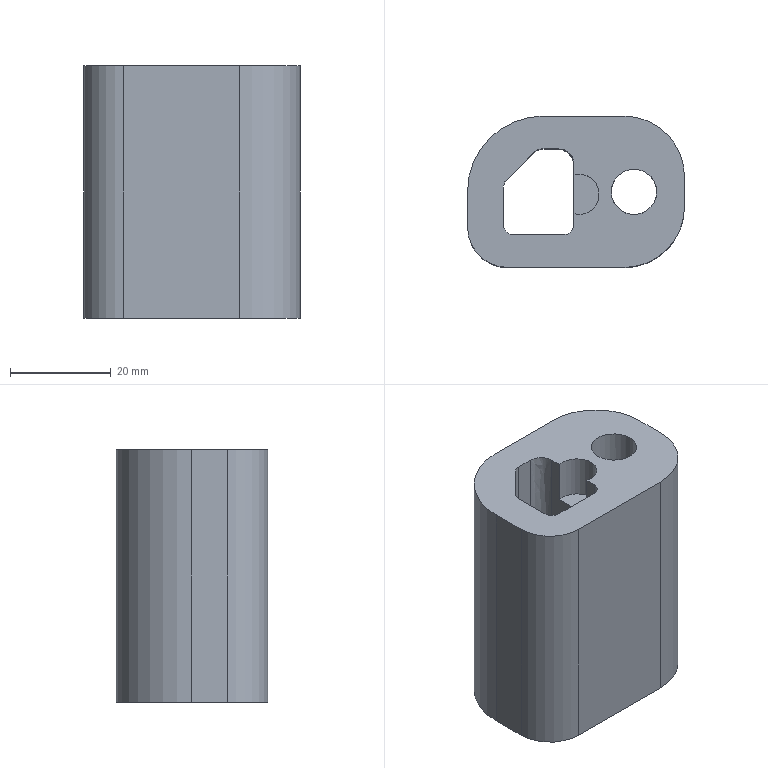Part | STEP file | PN_0018_id894_x_t | 1 solid | 25 faces | box 43 x 30 x 50 mm | volume 41594 mm3 | plane 13 | cylinder 10 | other 2 | commonest cylinder face diameters 4 x3 24 x2 8 x1 9 x1 14 x1 16 x1
STEP:
#1=CARTESIAN_POINT('',(-194.5,-101.127,86.5));
#2=VERTEX_POINT('',#1);
#3=CARTESIAN_POINT('',(-194.5,-108.873,86.5));
#4=VERTEX_POINT('',#3);
#5=CARTESIAN_POINT('',(-194.5,-99.,86.5));
#6=DIRECTION('',(0.,-1.,0.));
#7=VECTOR('',#6,1.);
#8=LINE('',#5,#7);
#9=EDGE_CURVE('',#2,#4,#8,.T.);
#10=ORIENTED_EDGE('',*,*,#9,.F.);
#11=CARTESIAN_POINT('',(-194.5,-101.127,95.));
#12=VERTEX_POINT('',#11);
#13=CARTESIAN_POINT('',(-194.5,-101.127,86.5));
#14=DIRECTION('',(0.,0.,1.));
#15=VECTOR('',#14,1.);
#16=LINE('',#13,#15);
#17=EDGE_CURVE('',#2,#12,#16,.T.);
#18=ORIENTED_EDGE('',*,*,#17,.T.);
#19=CARTESIAN_POINT('',(-194.5,-99.,95.));
#20=VERTEX_POINT('',#19);
#21=CARTESIAN_POINT('',(-194.5,-99.,95.));
#22=DIRECTION('',(0.,-1.,0.));
#23=VECTOR('',#22,1.);
#24=LINE('',#21,#23);
#25=EDGE_CURVE('',#20,#12,#24,.T.);
#26=ORIENTED_EDGE('',*,*,#25,.F.);
#27=CARTESIAN_POINT('',(-194.5,-99.,45.));
#28=VERTEX_POINT('',#27);
#29=CARTESIAN_POINT('',(-194.5,-99.,78.6));
#30=DIRECTION('',(0.,0.,-1.));
#31=VECTOR('',#30,1.);
#32=LINE('',#29,#31);
#33=EDGE_CURVE('',#20,#28,#32,.T.);
#34=ORIENTED_EDGE('',*,*,#33,.T.);
#35=CARTESIAN_POINT('',(-194.5,-111.,45.));
#36=VERTEX_POINT('',#35);
#37=CARTESIAN_POINT('',(-194.5,-99.,45.));
#38=DIRECTION('',(0.,-1.,0.));
#39=VECTOR('',#38,1.);
#40=LINE('',#37,#39);
#41=EDGE_CURVE('',#28,#36,#40,.T.);
#42=ORIENTED_EDGE('',*,*,#41,.T.);
#43=CARTESIAN_POINT('',(-194.5,-111.,95.));
#44=VERTEX_POINT('',#43);
#45=CARTESIAN_POINT('',(-194.5,-111.,78.6));
#46=DIRECTION('',(0.,0.,-1.));
#47=VECTOR('',#46,1.);
#48=LINE('',#45,#47);
#49=EDGE_CURVE('',#44,#36,#48,.T.);
#50=ORIENTED_EDGE('',*,*,#49,.F.);
#51=CARTESIAN_POINT('',(-194.5,-108.873,95.));
#52=VERTEX_POINT('',#51);
#53=CARTESIAN_POINT('',(-194.5,-99.,95.));
#54=DIRECTION('',(0.,-1.,0.));
#55=VECTOR('',#54,1.);
#56=LINE('',#53,#55);
#57=EDGE_CURVE('',#52,#44,#56,.T.);
#58=ORIENTED_EDGE('',*,*,#57,.F.);
#59=CARTESIAN_POINT('',(-194.5,-108.873,86.5));
#60=DIRECTION('',(0.,0.,-1.));
#61=VECTOR('',#60,1.);
#62=LINE('',#59,#61);
#63=EDGE_CURVE('',#52,#4,#62,.T.);
#64=ORIENTED_EDGE('',*,*,#63,.T.);
#65=EDGE_LOOP('',(#10,#18,#26,#34,#42,#50,#58,#64));
#66=FACE_OUTER_BOUND('',#65,.T.);
#67=CARTESIAN_POINT('',(-194.5,-99.,78.6));
#68=DIRECTION('',(1.,0.,0.));
#69=DIRECTION('',(0.,0.,-1.));
#70=AXIS2_PLACEMENT_3D('',#67,#68,#69);
#71=PLANE('',#70);
#72=ADVANCED_FACE('',(#66),#71,.F.);
#73=CARTESIAN_POINT('',(-187.086,-104.5,95.));
#74=VERTEX_POINT('',#73);
#75=CARTESIAN_POINT('',(-182.586,-104.5,95.));
#76=DIRECTION('',(0.,0.,1.));
#77=DIRECTION('',(-1.,0.,0.));
#78=AXIS2_PLACEMENT_3D('',#75,#76,#77);
#79=CIRCLE('',#78,4.5);
#80=EDGE_CURVE('',#74,#74,#79,.T.);
#81=ORIENTED_EDGE('',*,*,#80,.F.);
#82=EDGE_LOOP('',(#81));
#83=FACE_BOUND('',#82,.T.);
#84=CARTESIAN_POINT('',(-193.5,-105.,95.));
#85=DIRECTION('',(0.,0.,1.));
#86=DIRECTION('',(1.,0.,0.));
#87=AXIS2_PLACEMENT_3D('',#84,#85,#86);
#88=CIRCLE('',#87,4.);
#89=EDGE_CURVE('',#52,#12,#88,.T.);
#90=ORIENTED_EDGE('',*,*,#89,.F.);
#91=ORIENTED_EDGE('',*,*,#57,.T.);
#92=CARTESIAN_POINT('',(-196.5,-113.,95.));
#93=VERTEX_POINT('',#92);
#94=CARTESIAN_POINT('',(-196.5,-111.,95.));
#95=DIRECTION('',(0.,0.,-1.));
#96=DIRECTION('',(-1.,0.,0.));
#97=AXIS2_PLACEMENT_3D('',#94,#95,#96);
#98=CIRCLE('',#97,2.);
#99=EDGE_CURVE('',#44,#93,#98,.T.);
#100=ORIENTED_EDGE('',*,*,#99,.T.);
#101=CARTESIAN_POINT('',(-206.5,-113.,95.));
#102=VERTEX_POINT('',#101);
#103=CARTESIAN_POINT('',(-196.5,-113.,95.));
#104=DIRECTION('',(-1.,0.,0.));
#105=VECTOR('',#104,1.);
#106=LINE('',#103,#105);
#107=EDGE_CURVE('',#93,#102,#106,.T.);
#108=ORIENTED_EDGE('',*,*,#107,.T.);
#109=CARTESIAN_POINT('',(-208.5,-111.,95.));
#110=VERTEX_POINT('',#109);
#111=CARTESIAN_POINT('',(-206.5,-111.,95.));
#112=DIRECTION('',(0.,0.,-1.));
#113=DIRECTION('',(-1.,0.,0.));
#114=AXIS2_PLACEMENT_3D('',#111,#112,#113);
#115=CIRCLE('',#114,2.);
#116=EDGE_CURVE('',#102,#110,#115,.T.);
#117=ORIENTED_EDGE('',*,*,#116,.T.);
#118=CARTESIAN_POINT('',(-208.5,-103.657,95.));
#119=VERTEX_POINT('',#118);
#120=CARTESIAN_POINT('',(-208.5,-111.,95.));
#121=DIRECTION('',(0.,1.,0.));
#122=VECTOR('',#121,1.);
#123=LINE('',#120,#122);
#124=EDGE_CURVE('',#110,#119,#123,.T.);
#125=ORIENTED_EDGE('',*,*,#124,.T.);
#126=CARTESIAN_POINT('',(-207.914,-102.243,95.));
#127=VERTEX_POINT('',#126);
#128=CARTESIAN_POINT('',(-206.5,-103.657,95.));
#129=DIRECTION('',(0.,0.,-1.));
#130=DIRECTION('',(-1.,0.,0.));
#131=AXIS2_PLACEMENT_3D('',#128,#129,#130);
#132=CIRCLE('',#131,2.);
#133=EDGE_CURVE('',#119,#127,#132,.T.);
#134=ORIENTED_EDGE('',*,*,#133,.T.);
#135=CARTESIAN_POINT('',(-202.257,-96.586,95.));
#136=VERTEX_POINT('',#135);
#137=CARTESIAN_POINT('',(-207.914,-102.243,95.));
#138=DIRECTION('',(0.7071,0.7071,0.));
#139=VECTOR('',#138,1.);
#140=LINE('',#137,#139);
#141=EDGE_CURVE('',#127,#136,#140,.T.);
#142=ORIENTED_EDGE('',*,*,#141,.T.);
#143=CARTESIAN_POINT('',(-200.843,-96.,95.));
#144=VERTEX_POINT('',#143);
#145=CARTESIAN_POINT('',(-202.257,-96.586,95.));
#146=CARTESIAN_POINT('',(-201.885,-96.213,95.));
#147=CARTESIAN_POINT('',(-201.37,-96.,95.));
#148=CARTESIAN_POINT('',(-200.843,-96.,95.));
#149=B_SPLINE_CURVE_WITH_KNOTS('',3,(#145,#146,#147,#148),.UNSPECIFIED.,.F.,.F.,(4,4),(0.,1.),.UNSPECIFIED.);
#150=EDGE_CURVE('',#136,#144,#149,.T.);
#151=ORIENTED_EDGE('',*,*,#150,.T.);
#152=CARTESIAN_POINT('',(-197.5,-96.,95.));
#153=VERTEX_POINT('',#152);
#154=CARTESIAN_POINT('',(-200.843,-96.,95.));
#155=DIRECTION('',(1.,0.,0.));
#156=VECTOR('',#155,1.);
#157=LINE('',#154,#156);
#158=EDGE_CURVE('',#144,#153,#157,.T.);
#159=ORIENTED_EDGE('',*,*,#158,.T.);
#160=CARTESIAN_POINT('',(-197.5,-96.,95.));
#161=CARTESIAN_POINT('',(-196.717,-96.,95.));
#162=CARTESIAN_POINT('',(-195.94,-96.317,95.));
#163=CARTESIAN_POINT('',(-194.817,-97.441,95.));
#164=CARTESIAN_POINT('',(-194.5,-98.203,95.));
#165=CARTESIAN_POINT('',(-194.5,-99.,95.));
#166=B_SPLINE_CURVE_WITH_KNOTS('',3,(#160,#161,#162,#163,#164,#165),.UNSPECIFIED.,.F.,.F.,(4,2,4),(0.,0.5,1.),.UNSPECIFIED.);
#167=EDGE_CURVE('',#153,#20,#166,.T.);
#168=ORIENTED_EDGE('',*,*,#167,.T.);
#169=ORIENTED_EDGE('',*,*,#25,.T.);
#170=EDGE_LOOP('',(#90,#91,#100,#108,#117,#125,#134,#142,#151,#159,#168,#169));
#171=FACE_BOUND('',#170,.T.);
#172=CARTESIAN_POINT('',(-215.586,-104.5,95.));
#173=VERTEX_POINT('',#172);
#174=CARTESIAN_POINT('',(-215.586,-111.5,95.));
#175=VERTEX_POINT('',#174);
#176=CARTESIAN_POINT('',(-215.586,-80.,95.));
#177=DIRECTION('',(0.,-1.,0.));
#178=VECTOR('',#177,1.);
#179=LINE('',#176,#178);
#180=EDGE_CURVE('',#173,#175,#179,.T.);
#181=ORIENTED_EDGE('',*,*,#180,.T.);
#182=CARTESIAN_POINT('',(-207.586,-119.5,95.));
#183=VERTEX_POINT('',#182);
#184=CARTESIAN_POINT('',(-207.586,-111.5,95.));
#185=DIRECTION('',(0.,0.,1.));
#186=DIRECTION('',(-1.,0.,0.));
#187=AXIS2_PLACEMENT_3D('',#184,#185,#186);
#188=CIRCLE('',#187,8.);
#189=EDGE_CURVE('',#175,#183,#188,.T.);
#190=ORIENTED_EDGE('',*,*,#189,.T.);
#191=CARTESIAN_POINT('',(-184.586,-119.5,95.));
#192=VERTEX_POINT('',#191);
#193=CARTESIAN_POINT('',(-211.586,-119.5,95.));
#194=DIRECTION('',(1.,0.,0.));
#195=VECTOR('',#194,1.);
#196=LINE('',#193,#195);
#197=EDGE_CURVE('',#183,#192,#196,.T.);
#198=ORIENTED_EDGE('',*,*,#197,.T.);
#199=CARTESIAN_POINT('',(-172.586,-107.5,95.));
#200=VERTEX_POINT('',#199);
#201=CARTESIAN_POINT('',(-184.586,-107.5,95.));
#202=DIRECTION('',(0.,0.,1.));
#203=DIRECTION('',(-1.,0.,0.));
#204=AXIS2_PLACEMENT_3D('',#201,#202,#203);
#205=CIRCLE('',#204,12.);
#206=EDGE_CURVE('',#192,#200,#205,.T.);
#207=ORIENTED_EDGE('',*,*,#206,.T.);
#208=CARTESIAN_POINT('',(-172.586,-101.5,95.));
#209=VERTEX_POINT('',#208);
#210=CARTESIAN_POINT('',(-172.586,-115.,95.));
#211=DIRECTION('',(0.,1.,0.));
#212=VECTOR('',#211,1.);
#213=LINE('',#210,#212);
#214=EDGE_CURVE('',#200,#209,#213,.T.);
#215=ORIENTED_EDGE('',*,*,#214,.T.);
#216=CARTESIAN_POINT('',(-184.586,-89.5,95.));
#217=VERTEX_POINT('',#216);
#218=CARTESIAN_POINT('',(-184.586,-101.5,95.));
#219=DIRECTION('',(0.,0.,1.));
#220=DIRECTION('',(-1.,0.,0.));
#221=AXIS2_PLACEMENT_3D('',#218,#219,#220);
#222=CIRCLE('',#221,12.);
#223=EDGE_CURVE('',#209,#217,#222,.T.);
#224=ORIENTED_EDGE('',*,*,#223,.T.);
#225=CARTESIAN_POINT('',(-200.586,-89.5,95.));
#226=VERTEX_POINT('',#225);
#227=CARTESIAN_POINT('',(-189.586,-89.5,95.));
#228=DIRECTION('',(-1.,0.,0.));
#229=VECTOR('',#228,1.);
#230=LINE('',#227,#229);
#231=EDGE_CURVE('',#217,#226,#230,.T.);
#232=ORIENTED_EDGE('',*,*,#231,.T.);
#233=CARTESIAN_POINT('',(-200.586,-104.5,95.));
#234=DIRECTION('',(0.,0.,1.));
#235=DIRECTION('',(-1.,0.,0.));
#236=AXIS2_PLACEMENT_3D('',#233,#234,#235);
#237=CIRCLE('',#236,15.);
#238=EDGE_CURVE('',#226,#173,#237,.T.);
#239=ORIENTED_EDGE('',*,*,#238,.T.);
#240=EDGE_LOOP('',(#181,#190,#198,#207,#215,#224,#232,#239));
#241=FACE_BOUND('',#240,.T.);
#242=CARTESIAN_POINT('',(-114.973,24.687,95.));
#243=DIRECTION('',(0.,0.,-1.));
#244=DIRECTION('',(-1.,0.,0.));
#245=AXIS2_PLACEMENT_3D('',#242,#243,#244);
#246=PLANE('',#245);
#247=ADVANCED_FACE('',(#83,#171,#241),#246,.F.);
#248=CARTESIAN_POINT('',(-215.586,-111.5,45.));
#249=VERTEX_POINT('',#248);
#250=CARTESIAN_POINT('',(-215.586,-104.5,45.));
#251=VERTEX_POINT('',#250);
#252=CARTESIAN_POINT('',(-215.586,-64.,45.));
#253=DIRECTION('',(0.,1.,0.));
#254=VECTOR('',#253,1.);
#255=LINE('',#252,#254);
#256=EDGE_CURVE('',#249,#251,#255,.T.);
#257=ORIENTED_EDGE('',*,*,#256,.F.);
#258=CARTESIAN_POINT('',(-215.586,-111.5,78.6));
#259=DIRECTION('',(0.,0.,1.));
#260=VECTOR('',#259,1.);
#261=LINE('',#258,#260);
#262=EDGE_CURVE('',#249,#175,#261,.T.);
#263=ORIENTED_EDGE('',*,*,#262,.T.);
#264=ORIENTED_EDGE('',*,*,#180,.F.);
#265=CARTESIAN_POINT('',(-215.586,-104.5,78.6));
#266=DIRECTION('',(0.,0.,-1.));
#267=VECTOR('',#266,1.);
#268=LINE('',#265,#267);
#269=EDGE_CURVE('',#173,#251,#268,.T.);
#270=ORIENTED_EDGE('',*,*,#269,.T.);
#271=EDGE_LOOP('',(#257,#263,#264,#270));
#272=FACE_OUTER_BOUND('',#271,.T.);
#273=CARTESIAN_POINT('',(-215.586,-80.,78.6));
#274=DIRECTION('',(1.,0.,0.));
#275=DIRECTION('',(0.,0.,-1.));
#276=AXIS2_PLACEMENT_3D('',#273,#274,#275);
#277=PLANE('',#276);
#278=ADVANCED_FACE('',(#272),#277,.F.);
#279=ORIENTED_EDGE('',*,*,#197,.F.);
#280=CARTESIAN_POINT('',(-207.586,-119.5,45.));
#281=VERTEX_POINT('',#280);
#282=CARTESIAN_POINT('',(-207.586,-119.5,78.6));
#283=DIRECTION('',(0.,0.,-1.));
#284=VECTOR('',#283,1.);
#285=LINE('',#282,#284);
#286=EDGE_CURVE('',#183,#281,#285,.T.);
#287=ORIENTED_EDGE('',*,*,#286,.T.);
#288=CARTESIAN_POINT('',(-184.586,-119.5,45.));
#289=VERTEX_POINT('',#288);
#290=CARTESIAN_POINT('',(-211.586,-119.5,45.));
#291=DIRECTION('',(1.,0.,0.));
#292=VECTOR('',#291,1.);
#293=LINE('',#290,#292);
#294=EDGE_CURVE('',#281,#289,#293,.T.);
#295=ORIENTED_EDGE('',*,*,#294,.T.);
#296=CARTESIAN_POINT('',(-184.586,-119.5,78.6));
#297=DIRECTION('',(0.,0.,1.));
#298=VECTOR('',#297,1.);
#299=LINE('',#296,#298);
#300=EDGE_CURVE('',#289,#192,#299,.T.);
#301=ORIENTED_EDGE('',*,*,#300,.T.);
#302=EDGE_LOOP('',(#279,#287,#295,#301));
#303=FACE_OUTER_BOUND('',#302,.T.);
#304=CARTESIAN_POINT('',(-211.586,-119.5,78.6));
#305=DIRECTION('',(0.,1.,0.));
#306=DIRECTION('',(0.,0.,1.));
#307=AXIS2_PLACEMENT_3D('',#304,#305,#306);
#308=PLANE('',#307);
#309=ADVANCED_FACE('',(#303),#308,.F.);
#310=ORIENTED_EDGE('',*,*,#214,.F.);
#311=CARTESIAN_POINT('',(-172.586,-107.5,45.));
#312=VERTEX_POINT('',#311);
#313=CARTESIAN_POINT('',(-172.586,-107.5,78.6));
#314=DIRECTION('',(0.,0.,-1.));
#315=VECTOR('',#314,1.);
#316=LINE('',#313,#315);
#317=EDGE_CURVE('',#200,#312,#316,.T.);
#318=ORIENTED_EDGE('',*,*,#317,.T.);
#319=CARTESIAN_POINT('',(-172.586,-101.5,45.));
#320=VERTEX_POINT('',#319);
#321=CARTESIAN_POINT('',(-172.586,-115.,45.));
#322=DIRECTION('',(0.,1.,0.));
#323=VECTOR('',#322,1.);
#324=LINE('',#321,#323);
#325=EDGE_CURVE('',#312,#320,#324,.T.);
#326=ORIENTED_EDGE('',*,*,#325,.T.);
#327=CARTESIAN_POINT('',(-172.586,-101.5,78.6));
#328=DIRECTION('',(0.,0.,1.));
#329=VECTOR('',#328,1.);
#330=LINE('',#327,#329);
#331=EDGE_CURVE('',#320,#209,#330,.T.);
#332=ORIENTED_EDGE('',*,*,#331,.T.);
#333=EDGE_LOOP('',(#310,#318,#326,#332));
#334=FACE_OUTER_BOUND('',#333,.T.);
#335=CARTESIAN_POINT('',(-172.586,-115.,78.6));
#336=DIRECTION('',(-1.,0.,0.));
#337=DIRECTION('',(0.,0.,1.));
#338=AXIS2_PLACEMENT_3D('',#335,#336,#337);
#339=PLANE('',#338);
#340=ADVANCED_FACE('',(#334),#339,.F.);
#341=CARTESIAN_POINT('',(-200.586,-89.5,45.));
#342=VERTEX_POINT('',#341);
#343=CARTESIAN_POINT('',(-184.586,-89.5,45.));
#344=VERTEX_POINT('',#343);
#345=CARTESIAN_POINT('',(-119.811,-89.5,45.));
#346=DIRECTION('',(1.,0.,0.));
#347=VECTOR('',#346,1.);
#348=LINE('',#345,#347);
#349=EDGE_CURVE('',#342,#344,#348,.T.);
#350=ORIENTED_EDGE('',*,*,#349,.F.);
#351=CARTESIAN_POINT('',(-200.586,-89.5,78.6));
#352=DIRECTION('',(0.,0.,1.));
#353=VECTOR('',#352,1.);
#354=LINE('',#351,#353);
#355=EDGE_CURVE('',#342,#226,#354,.T.);
#356=ORIENTED_EDGE('',*,*,#355,.T.);
#357=ORIENTED_EDGE('',*,*,#231,.F.);
#358=CARTESIAN_POINT('',(-184.586,-89.5,78.6));
#359=DIRECTION('',(0.,0.,-1.));
#360=VECTOR('',#359,1.);
#361=LINE('',#358,#360);
#362=EDGE_CURVE('',#217,#344,#361,.T.);
#363=ORIENTED_EDGE('',*,*,#362,.T.);
#364=EDGE_LOOP('',(#350,#356,#357,#363));
#365=FACE_OUTER_BOUND('',#364,.T.);
#366=CARTESIAN_POINT('',(-189.586,-89.5,78.6));
#367=DIRECTION('',(0.,-1.,0.));
#368=DIRECTION('',(0.,0.,-1.));
#369=AXIS2_PLACEMENT_3D('',#366,#367,#368);
#370=PLANE('',#369);
#371=ADVANCED_FACE('',(#365),#370,.F.);
#372=CARTESIAN_POINT('',(-182.586,-111.5,45.));
#373=VERTEX_POINT('',#372);
#374=CARTESIAN_POINT('',(-182.586,-104.5,45.));
#375=DIRECTION('',(0.,0.,1.));
#376=DIRECTION('',(0.,-1.,0.));
#377=AXIS2_PLACEMENT_3D('',#374,#375,#376);
#378=CIRCLE('',#377,7.);
#379=EDGE_CURVE('',#373,#373,#378,.T.);
#380=ORIENTED_EDGE('',*,*,#379,.T.);
#381=EDGE_LOOP('',(#380));
#382=FACE_BOUND('',#381,.T.);
#383=CARTESIAN_POINT('',(-206.5,-113.,45.));
#384=VERTEX_POINT('',#383);
#385=CARTESIAN_POINT('',(-208.5,-111.,45.));
#386=VERTEX_POINT('',#385);
#387=CARTESIAN_POINT('',(-206.5,-111.,45.));
#388=DIRECTION('',(0.,0.,-1.));
#389=DIRECTION('',(1.,0.,0.));
#390=AXIS2_PLACEMENT_3D('',#387,#388,#389);
#391=CIRCLE('',#390,2.);
#392=EDGE_CURVE('',#384,#386,#391,.T.);
#393=ORIENTED_EDGE('',*,*,#392,.F.);
#394=CARTESIAN_POINT('',(-196.5,-113.,45.));
#395=VERTEX_POINT('',#394);
#396=CARTESIAN_POINT('',(-119.811,-113.,45.));
#397=DIRECTION('',(1.,0.,0.));
#398=VECTOR('',#397,1.);
#399=LINE('',#396,#398);
#400=EDGE_CURVE('',#384,#395,#399,.T.);
#401=ORIENTED_EDGE('',*,*,#400,.T.);
#402=CARTESIAN_POINT('',(-196.5,-111.,45.));
#403=DIRECTION('',(0.,0.,1.));
#404=DIRECTION('',(1.,0.,0.));
#405=AXIS2_PLACEMENT_3D('',#402,#403,#404);
#406=CIRCLE('',#405,2.);
#407=EDGE_CURVE('',#395,#36,#406,.T.);
#408=ORIENTED_EDGE('',*,*,#407,.T.);
#409=ORIENTED_EDGE('',*,*,#41,.F.);
#410=CARTESIAN_POINT('',(-197.5,-96.,45.));
#411=VERTEX_POINT('',#410);
#412=CARTESIAN_POINT('',(-194.5,-99.,45.));
#413=CARTESIAN_POINT('',(-194.5,-98.664,45.));
#414=CARTESIAN_POINT('',(-194.558,-98.324,45.));
#415=CARTESIAN_POINT('',(-194.669,-98.008,45.));
#416=CARTESIAN_POINT('',(-194.78,-97.691,45.));
#417=CARTESIAN_POINT('',(-194.947,-97.389,45.));
#418=CARTESIAN_POINT('',(-195.156,-97.127,45.));
#419=CARTESIAN_POINT('',(-195.366,-96.864,45.));
#420=CARTESIAN_POINT('',(-195.626,-96.635,45.));
#421=CARTESIAN_POINT('',(-195.912,-96.458,45.));
#422=CARTESIAN_POINT('',(-196.193,-96.284,45.));
#423=CARTESIAN_POINT('',(-196.506,-96.154,45.));
#424=CARTESIAN_POINT('',(-196.828,-96.079,45.));
#425=CARTESIAN_POINT('',(-197.048,-96.027,45.));
#426=CARTESIAN_POINT('',(-197.275,-96.,45.));
#427=CARTESIAN_POINT('',(-197.5,-96.,45.));
#428=B_SPLINE_CURVE_WITH_KNOTS('',3,(#412,#413,#414,#415,#416,#417,#418,#419,#420,#421,#422,#423,#424,#425,#426,#427),.UNSPECIFIED.,.F.,.F.,(4,3,3,3,3,4),(0.,0.2148,0.4297,0.6453,0.8567,1.),.UNSPECIFIED.);
#429=EDGE_CURVE('',#28,#411,#428,.T.);
#430=ORIENTED_EDGE('',*,*,#429,.T.);
#431=CARTESIAN_POINT('',(-200.843,-96.,45.));
#432=VERTEX_POINT('',#431);
#433=CARTESIAN_POINT('',(-119.811,-96.,45.));
#434=DIRECTION('',(-1.,0.,0.));
#435=VECTOR('',#434,1.);
#436=LINE('',#433,#435);
#437=EDGE_CURVE('',#411,#432,#436,.T.);
#438=ORIENTED_EDGE('',*,*,#437,.T.);
#439=CARTESIAN_POINT('',(-202.257,-96.586,45.));
#440=VERTEX_POINT('',#439);
#441=CARTESIAN_POINT('',(-200.843,-96.,45.));
#442=CARTESIAN_POINT('',(-200.983,-96.,45.));
#443=CARTESIAN_POINT('',(-201.124,-96.015,45.));
#444=CARTESIAN_POINT('',(-201.261,-96.045,45.));
#445=CARTESIAN_POINT('',(-201.482,-96.093,45.));
#446=CARTESIAN_POINT('',(-201.699,-96.179,45.));
#447=CARTESIAN_POINT('',(-201.891,-96.298,45.));
#448=CARTESIAN_POINT('',(-202.024,-96.379,45.));
#449=CARTESIAN_POINT('',(-202.148,-96.476,45.));
#450=CARTESIAN_POINT('',(-202.257,-96.586,45.));
#451=B_SPLINE_CURVE_WITH_KNOTS('',3,(#441,#442,#443,#444,#445,#446,#447,#448,#449,#450),.UNSPECIFIED.,.F.,.F.,(4,3,3,4),(0.,0.2675,0.7033,1.),.UNSPECIFIED.);
#452=EDGE_CURVE('',#432,#440,#451,.T.);
#453=ORIENTED_EDGE('',*,*,#452,.T.);
#454=CARTESIAN_POINT('',(-207.914,-102.243,45.));
#455=VERTEX_POINT('',#454);
#456=CARTESIAN_POINT('',(-144.741,-39.069,45.));
#457=DIRECTION('',(-0.7071,-0.7071,0.));
#458=VECTOR('',#457,1.);
#459=LINE('',#456,#458);
#460=EDGE_CURVE('',#440,#455,#459,.T.);
#461=ORIENTED_EDGE('',*,*,#460,.T.);
#462=CARTESIAN_POINT('',(-208.5,-103.657,45.));
#463=VERTEX_POINT('',#462);
#464=CARTESIAN_POINT('',(-206.5,-103.657,45.));
#465=DIRECTION('',(0.,0.,-1.));
#466=DIRECTION('',(1.,0.,0.));
#467=AXIS2_PLACEMENT_3D('',#464,#465,#466);
#468=CIRCLE('',#467,2.);
#469=EDGE_CURVE('',#463,#455,#468,.T.);
#470=ORIENTED_EDGE('',*,*,#469,.F.);
#471=CARTESIAN_POINT('',(-208.5,-64.,45.));
#472=DIRECTION('',(0.,-1.,0.));
#473=VECTOR('',#472,1.);
#474=LINE('',#471,#473);
#475=EDGE_CURVE('',#463,#386,#474,.T.);
#476=ORIENTED_EDGE('',*,*,#475,.T.);
#477=EDGE_LOOP('',(#393,#401,#408,#409,#430,#438,#453,#461,#470,#476));
#478=FACE_BOUND('',#477,.T.);
#479=ORIENTED_EDGE('',*,*,#294,.F.);
#480=CARTESIAN_POINT('',(-207.586,-111.5,45.));
#481=DIRECTION('',(0.,0.,-1.));
#482=DIRECTION('',(1.,0.,0.));
#483=AXIS2_PLACEMENT_3D('',#480,#481,#482);
#484=CIRCLE('',#483,8.);
#485=EDGE_CURVE('',#281,#249,#484,.T.);
#486=ORIENTED_EDGE('',*,*,#485,.T.);
#487=ORIENTED_EDGE('',*,*,#256,.T.);
#488=CARTESIAN_POINT('',(-200.586,-104.5,45.));
#489=DIRECTION('',(0.,0.,-1.));
#490=DIRECTION('',(1.,0.,0.));
#491=AXIS2_PLACEMENT_3D('',#488,#489,#490);
#492=CIRCLE('',#491,15.);
#493=EDGE_CURVE('',#251,#342,#492,.T.);
#494=ORIENTED_EDGE('',*,*,#493,.T.);
#495=ORIENTED_EDGE('',*,*,#349,.T.);
#496=CARTESIAN_POINT('',(-184.586,-101.5,45.));
#497=DIRECTION('',(0.,0.,-1.));
#498=DIRECTION('',(1.,0.,0.));
#499=AXIS2_PLACEMENT_3D('',#496,#497,#498);
#500=CIRCLE('',#499,12.);
#501=EDGE_CURVE('',#344,#320,#500,.T.);
#502=ORIENTED_EDGE('',*,*,#501,.T.);
#503=ORIENTED_EDGE('',*,*,#325,.F.);
#504=CARTESIAN_POINT('',(-184.586,-107.5,45.));
#505=DIRECTION('',(0.,0.,-1.));
#506=DIRECTION('',(1.,0.,0.));
#507=AXIS2_PLACEMENT_3D('',#504,#505,#506);
#508=CIRCLE('',#507,12.);
#509=EDGE_CURVE('',#312,#289,#508,.T.);
#510=ORIENTED_EDGE('',*,*,#509,.T.);
#511=EDGE_LOOP('',(#479,#486,#487,#494,#495,#502,#503,#510));
#512=FACE_BOUND('',#511,.T.);
#513=CARTESIAN_POINT('',(-119.811,-64.,45.));
#514=DIRECTION('',(0.,0.,1.));
#515=DIRECTION('',(1.,0.,0.));
#516=AXIS2_PLACEMENT_3D('',#513,#514,#515);
#517=PLANE('',#516);
#518=ADVANCED_FACE('',(#382,#478,#512),#517,.F.);
#519=ORIENTED_EDGE('',*,*,#475,.F.);
#520=CARTESIAN_POINT('',(-208.5,-103.657,78.6));
#521=DIRECTION('',(0.,0.,-1.));
#522=VECTOR('',#521,1.);
#523=LINE('',#520,#522);
#524=EDGE_CURVE('',#119,#463,#523,.T.);
#525=ORIENTED_EDGE('',*,*,#524,.F.);
#526=ORIENTED_EDGE('',*,*,#124,.F.);
#527=CARTESIAN_POINT('',(-208.5,-111.,78.6));
#528=DIRECTION('',(0.,0.,-1.));
#529=VECTOR('',#528,1.);
#530=LINE('',#527,#529);
#531=EDGE_CURVE('',#110,#386,#530,.T.);
#532=ORIENTED_EDGE('',*,*,#531,.T.);
#533=EDGE_LOOP('',(#519,#525,#526,#532));
#534=FACE_OUTER_BOUND('',#533,.T.);
#535=CARTESIAN_POINT('',(-208.5,-111.,78.6));
#536=DIRECTION('',(-1.,0.,0.));
#537=DIRECTION('',(0.,0.,1.));
#538=AXIS2_PLACEMENT_3D('',#535,#536,#537);
#539=PLANE('',#538);
#540=ADVANCED_FACE('',(#534),#539,.F.);
#541=ORIENTED_EDGE('',*,*,#469,.T.);
#542=CARTESIAN_POINT('',(-207.914,-102.243,78.6));
#543=DIRECTION('',(0.,0.,-1.));
#544=VECTOR('',#543,1.);
#545=LINE('',#542,#544);
#546=EDGE_CURVE('',#127,#455,#545,.T.);
#547=ORIENTED_EDGE('',*,*,#546,.F.);
#548=ORIENTED_EDGE('',*,*,#133,.F.);
#549=ORIENTED_EDGE('',*,*,#524,.T.);
#550=EDGE_LOOP('',(#541,#547,#548,#549));
#551=FACE_OUTER_BOUND('',#550,.T.);
#552=CARTESIAN_POINT('',(-206.5,-103.657,78.6));
#553=DIRECTION('',(0.,0.,-1.));
#554=DIRECTION('',(-1.,0.,0.));
#555=AXIS2_PLACEMENT_3D('',#552,#553,#554);
#556=CYLINDRICAL_SURFACE('',#555,2.);
#557=ADVANCED_FACE('',(#551),#556,.F.);
#558=ORIENTED_EDGE('',*,*,#546,.T.);
#559=ORIENTED_EDGE('',*,*,#460,.F.);
#560=CARTESIAN_POINT('',(-202.257,-96.586,78.6));
#561=DIRECTION('',(0.,0.,-1.));
#562=VECTOR('',#561,1.);
#563=LINE('',#560,#562);
#564=EDGE_CURVE('',#136,#440,#563,.T.);
#565=ORIENTED_EDGE('',*,*,#564,.F.);
#566=ORIENTED_EDGE('',*,*,#141,.F.);
#567=EDGE_LOOP('',(#558,#559,#565,#566));
#568=FACE_OUTER_BOUND('',#567,.T.);
#569=CARTESIAN_POINT('',(-207.914,-102.243,78.6));
#570=DIRECTION('',(-0.7071,0.7071,0.));
#571=DIRECTION('',(-0.7071,-0.7071,0.));
#572=AXIS2_PLACEMENT_3D('',#569,#570,#571);
#573=PLANE('',#572);
#574=ADVANCED_FACE('',(#568),#573,.F.);
#575=ORIENTED_EDGE('',*,*,#564,.T.);
#576=ORIENTED_EDGE('',*,*,#452,.F.);
#577=CARTESIAN_POINT('',(-200.843,-96.,78.6));
#578=DIRECTION('',(0.,0.,-1.));
#579=VECTOR('',#578,1.);
#580=LINE('',#577,#579);
#581=EDGE_CURVE('',#144,#432,#580,.T.);
#582=ORIENTED_EDGE('',*,*,#581,.F.);
#583=ORIENTED_EDGE('',*,*,#150,.F.);
#584=EDGE_LOOP('',(#575,#576,#582,#583));
#585=FACE_OUTER_BOUND('',#584,.T.);
#586=CARTESIAN_POINT('',(-202.257,-96.586,78.6));
#587=CARTESIAN_POINT('',(-201.885,-96.213,78.6));
#588=CARTESIAN_POINT('',(-201.37,-96.,78.6));
#589=CARTESIAN_POINT('',(-200.843,-96.,78.6));
#590=B_SPLINE_CURVE_WITH_KNOTS('',3,(#586,#587,#588,#589),.UNSPECIFIED.,.F.,.F.,(4,4),(0.,1.),.UNSPECIFIED.);
#591=DIRECTION('',(0.,0.,-1.));
#592=VECTOR('',#591,1.);
#593=SURFACE_OF_LINEAR_EXTRUSION('',#590,#592);
#594=ADVANCED_FACE('',(#585),#593,.F.);
#595=ORIENTED_EDGE('',*,*,#437,.F.);
#596=CARTESIAN_POINT('',(-197.5,-96.,78.6));
#597=DIRECTION('',(0.,0.,-1.));
#598=VECTOR('',#597,1.);
#599=LINE('',#596,#598);
#600=EDGE_CURVE('',#153,#411,#599,.T.);
#601=ORIENTED_EDGE('',*,*,#600,.F.);
#602=ORIENTED_EDGE('',*,*,#158,.F.);
#603=ORIENTED_EDGE('',*,*,#581,.T.);
#604=EDGE_LOOP('',(#595,#601,#602,#603));
#605=FACE_OUTER_BOUND('',#604,.T.);
#606=CARTESIAN_POINT('',(-200.843,-96.,78.6));
#607=DIRECTION('',(0.,1.,0.));
#608=DIRECTION('',(0.,0.,1.));
#609=AXIS2_PLACEMENT_3D('',#606,#607,#608);
#610=PLANE('',#609);
#611=ADVANCED_FACE('',(#605),#610,.F.);
#612=ORIENTED_EDGE('',*,*,#429,.F.);
#613=ORIENTED_EDGE('',*,*,#33,.F.);
#614=ORIENTED_EDGE('',*,*,#167,.F.);
#615=ORIENTED_EDGE('',*,*,#600,.T.);
#616=EDGE_LOOP('',(#612,#613,#614,#615));
#617=FACE_OUTER_BOUND('',#616,.T.);
#618=CARTESIAN_POINT('',(-197.5,-96.,78.6));
#619=CARTESIAN_POINT('',(-196.718,-96.,78.6));
#620=CARTESIAN_POINT('',(-195.933,-96.324,78.6));
#621=CARTESIAN_POINT('',(-195.102,-97.155,78.6));
#622=CARTESIAN_POINT('',(-194.879,-97.488,78.6));
#623=CARTESIAN_POINT('',(-194.578,-98.215,78.6));
#624=CARTESIAN_POINT('',(-194.5,-98.604,78.6));
#625=CARTESIAN_POINT('',(-194.5,-99.,78.6));
#626=B_SPLINE_CURVE_WITH_KNOTS('',3,(#618,#619,#620,#621,#622,#623,#624,#625),.UNSPECIFIED.,.F.,.F.,(4,2,2,4),(0.,0.5,0.75,1.),.UNSPECIFIED.);
#627=DIRECTION('',(0.,0.,-1.));
#628=VECTOR('',#627,1.);
#629=SURFACE_OF_LINEAR_EXTRUSION('',#626,#628);
#630=ADVANCED_FACE('',(#617),#629,.F.);
#631=ORIENTED_EDGE('',*,*,#49,.T.);
#632=ORIENTED_EDGE('',*,*,#407,.F.);
#633=CARTESIAN_POINT('',(-196.5,-113.,78.6));
#634=DIRECTION('',(0.,0.,-1.));
#635=VECTOR('',#634,1.);
#636=LINE('',#633,#635);
#637=EDGE_CURVE('',#93,#395,#636,.T.);
#638=ORIENTED_EDGE('',*,*,#637,.F.);
#639=ORIENTED_EDGE('',*,*,#99,.F.);
#640=EDGE_LOOP('',(#631,#632,#638,#639));
#641=FACE_OUTER_BOUND('',#640,.T.);
#642=CARTESIAN_POINT('',(-196.5,-111.,78.6));
#643=DIRECTION('',(0.,0.,-1.));
#644=DIRECTION('',(-1.,0.,0.));
#645=AXIS2_PLACEMENT_3D('',#642,#643,#644);
#646=CYLINDRICAL_SURFACE('',#645,2.);
#647=ADVANCED_FACE('',(#641),#646,.F.);
#648=ORIENTED_EDGE('',*,*,#400,.F.);
#649=CARTESIAN_POINT('',(-206.5,-113.,78.6));
#650=DIRECTION('',(0.,0.,-1.));
#651=VECTOR('',#650,1.);
#652=LINE('',#649,#651);
#653=EDGE_CURVE('',#102,#384,#652,.T.);
#654=ORIENTED_EDGE('',*,*,#653,.F.);
#655=ORIENTED_EDGE('',*,*,#107,.F.);
#656=ORIENTED_EDGE('',*,*,#637,.T.);
#657=EDGE_LOOP('',(#648,#654,#655,#656));
#658=FACE_OUTER_BOUND('',#657,.T.);
#659=CARTESIAN_POINT('',(-196.5,-113.,78.6));
#660=DIRECTION('',(0.,-1.,0.));
#661=DIRECTION('',(0.,0.,-1.));
#662=AXIS2_PLACEMENT_3D('',#659,#660,#661);
#663=PLANE('',#662);
#664=ADVANCED_FACE('',(#658),#663,.F.);
#665=ORIENTED_EDGE('',*,*,#653,.T.);
#666=ORIENTED_EDGE('',*,*,#392,.T.);
#667=ORIENTED_EDGE('',*,*,#531,.F.);
#668=ORIENTED_EDGE('',*,*,#116,.F.);
#669=EDGE_LOOP('',(#665,#666,#667,#668));
#670=FACE_OUTER_BOUND('',#669,.T.);
#671=CARTESIAN_POINT('',(-206.5,-111.,78.6));
#672=DIRECTION('',(0.,0.,-1.));
#673=DIRECTION('',(-1.,0.,0.));
#674=AXIS2_PLACEMENT_3D('',#671,#672,#673);
#675=CYLINDRICAL_SURFACE('',#674,2.);
#676=ADVANCED_FACE('',(#670),#675,.F.);
#677=ORIENTED_EDGE('',*,*,#9,.T.);
#678=CARTESIAN_POINT('',(-193.5,-105.,86.5));
#679=DIRECTION('',(0.,0.,-1.));
#680=DIRECTION('',(1.,0.,0.));
#681=AXIS2_PLACEMENT_3D('',#678,#679,#680);
#682=CIRCLE('',#681,4.);
#683=EDGE_CURVE('',#2,#4,#682,.T.);
#684=ORIENTED_EDGE('',*,*,#683,.F.);
#685=EDGE_LOOP('',(#677,#684));
#686=FACE_OUTER_BOUND('',#685,.T.);
#687=CARTESIAN_POINT('',(-193.5,-105.,86.5));
#688=DIRECTION('',(0.,0.,1.));
#689=DIRECTION('',(1.,0.,0.));
#690=AXIS2_PLACEMENT_3D('',#687,#688,#689);
#691=PLANE('',#690);
#692=ADVANCED_FACE('',(#686),#691,.T.);
#693=ORIENTED_EDGE('',*,*,#683,.T.);
#694=ORIENTED_EDGE('',*,*,#63,.F.);
#695=ORIENTED_EDGE('',*,*,#89,.T.);
#696=ORIENTED_EDGE('',*,*,#17,.F.);
#697=EDGE_LOOP('',(#693,#694,#695,#696));
#698=FACE_OUTER_BOUND('',#697,.T.);
#699=CARTESIAN_POINT('',(-193.5,-105.,86.5));
#700=DIRECTION('',(0.,0.,1.));
#701=DIRECTION('',(1.,0.,0.));
#702=AXIS2_PLACEMENT_3D('',#699,#700,#701);
#703=CYLINDRICAL_SURFACE('',#702,4.);
#704=ADVANCED_FACE('',(#698),#703,.F.);
#705=ORIENTED_EDGE('',*,*,#206,.F.);
#706=ORIENTED_EDGE('',*,*,#300,.F.);
#707=ORIENTED_EDGE('',*,*,#509,.F.);
#708=ORIENTED_EDGE('',*,*,#317,.F.);
#709=EDGE_LOOP('',(#705,#706,#707,#708));
#710=FACE_OUTER_BOUND('',#709,.T.);
#711=CARTESIAN_POINT('',(-184.586,-107.5,78.6));
#712=DIRECTION('',(0.,0.,-1.));
#713=DIRECTION('',(-1.,0.,0.));
#714=AXIS2_PLACEMENT_3D('',#711,#712,#713);
#715=CYLINDRICAL_SURFACE('',#714,12.);
#716=ADVANCED_FACE('',(#710),#715,.T.);
#717=ORIENTED_EDGE('',*,*,#223,.F.);
#718=ORIENTED_EDGE('',*,*,#331,.F.);
#719=ORIENTED_EDGE('',*,*,#501,.F.);
#720=ORIENTED_EDGE('',*,*,#362,.F.);
#721=EDGE_LOOP('',(#717,#718,#719,#720));
#722=FACE_OUTER_BOUND('',#721,.T.);
#723=CARTESIAN_POINT('',(-184.586,-101.5,78.6));
#724=DIRECTION('',(0.,0.,-1.));
#725=DIRECTION('',(-1.,0.,0.));
#726=AXIS2_PLACEMENT_3D('',#723,#724,#725);
#727=CYLINDRICAL_SURFACE('',#726,12.);
#728=ADVANCED_FACE('',(#722),#727,.T.);
#729=ORIENTED_EDGE('',*,*,#238,.F.);
#730=ORIENTED_EDGE('',*,*,#355,.F.);
#731=ORIENTED_EDGE('',*,*,#493,.F.);
#732=ORIENTED_EDGE('',*,*,#269,.F.);
#733=EDGE_LOOP('',(#729,#730,#731,#732));
#734=FACE_OUTER_BOUND('',#733,.T.);
#735=CARTESIAN_POINT('',(-200.586,-104.5,78.6));
#736=DIRECTION('',(0.,0.,-1.));
#737=DIRECTION('',(-1.,0.,0.));
#738=AXIS2_PLACEMENT_3D('',#735,#736,#737);
#739=CYLINDRICAL_SURFACE('',#738,15.);
#740=ADVANCED_FACE('',(#734),#739,.T.);
#741=ORIENTED_EDGE('',*,*,#485,.F.);
#742=ORIENTED_EDGE('',*,*,#286,.F.);
#743=ORIENTED_EDGE('',*,*,#189,.F.);
#744=ORIENTED_EDGE('',*,*,#262,.F.);
#745=EDGE_LOOP('',(#741,#742,#743,#744));
#746=FACE_OUTER_BOUND('',#745,.T.);
#747=CARTESIAN_POINT('',(-207.586,-111.5,78.6));
#748=DIRECTION('',(0.,0.,1.));
#749=DIRECTION('',(1.,0.,0.));
#750=AXIS2_PLACEMENT_3D('',#747,#748,#749);
#751=CYLINDRICAL_SURFACE('',#750,8.);
#752=ADVANCED_FACE('',(#746),#751,.T.);
#753=ORIENTED_EDGE('',*,*,#80,.T.);
#754=EDGE_LOOP('',(#753));
#755=FACE_BOUND('',#754,.T.);
#756=CARTESIAN_POINT('',(-182.586,-109.,75.));
#757=VERTEX_POINT('',#756);
#758=CARTESIAN_POINT('',(-182.586,-104.5,75.));
#759=DIRECTION('',(0.,0.,1.));
#760=DIRECTION('',(0.,-1.,0.));
#761=AXIS2_PLACEMENT_3D('',#758,#759,#760);
#762=CIRCLE('',#761,4.5);
#763=EDGE_CURVE('',#757,#757,#762,.T.);
#764=ORIENTED_EDGE('',*,*,#763,.F.);
#765=EDGE_LOOP('',(#764));
#766=FACE_BOUND('',#765,.T.);
#767=CARTESIAN_POINT('',(-182.586,-104.5,105.));
#768=DIRECTION('',(0.,0.,-1.));
#769=DIRECTION('',(0.,1.,0.));
#770=AXIS2_PLACEMENT_3D('',#767,#768,#769);
#771=CYLINDRICAL_SURFACE('',#770,4.5);
#772=ADVANCED_FACE('',(#755,#766),#771,.F.);
#773=ORIENTED_EDGE('',*,*,#763,.T.);
#774=EDGE_LOOP('',(#773));
#775=FACE_BOUND('',#774,.T.);
#776=CARTESIAN_POINT('',(-182.586,-97.5,75.));
#777=VERTEX_POINT('',#776);
#778=CARTESIAN_POINT('',(-182.586,-104.5,75.));
#779=DIRECTION('',(0.,0.,1.));
#780=DIRECTION('',(0.,1.,0.));
#781=AXIS2_PLACEMENT_3D('',#778,#779,#780);
#782=CIRCLE('',#781,7.);
#783=EDGE_CURVE('',#777,#777,#782,.T.);
#784=ORIENTED_EDGE('',*,*,#783,.F.);
#785=EDGE_LOOP('',(#784));
#786=FACE_BOUND('',#785,.T.);
#787=CARTESIAN_POINT('',(-182.586,-104.5,75.));
#788=DIRECTION('',(0.,0.,1.));
#789=DIRECTION('',(0.,-1.,0.));
#790=AXIS2_PLACEMENT_3D('',#787,#788,#789);
#791=PLANE('',#790);
#792=ADVANCED_FACE('',(#775,#786),#791,.F.);
#793=ORIENTED_EDGE('',*,*,#379,.F.);
#794=EDGE_LOOP('',(#793));
#795=FACE_BOUND('',#794,.T.);
#796=ORIENTED_EDGE('',*,*,#783,.T.);
#797=EDGE_LOOP('',(#796));
#798=FACE_BOUND('',#797,.T.);
#799=CARTESIAN_POINT('',(-182.586,-104.5,75.));
#800=DIRECTION('',(0.,0.,-1.));
#801=DIRECTION('',(0.,1.,0.));
#802=AXIS2_PLACEMENT_3D('',#799,#800,#801);
#803=CYLINDRICAL_SURFACE('',#802,7.);
#804=ADVANCED_FACE('',(#795,#798),#803,.F.);
#805=CLOSED_SHELL('',(#72,#247,#278,#309,#340,#371,#518,#540,#557,#574,#594,#611,#630,#647,#664,#676,#692,#704,#716,#728,#740,#752,#772,#792,#804));
#806=MANIFOLD_SOLID_BREP('',#805);
#807=(LENGTH_UNIT()NAMED_UNIT(*)SI_UNIT(.MILLI.,.METRE.));
#808=UNCERTAINTY_MEASURE_WITH_UNIT(LENGTH_MEASURE(0.0508),#807,'','');
#809=(NAMED_UNIT(*)PLANE_ANGLE_UNIT()SI_UNIT($,.RADIAN.));
#810=PLANE_ANGLE_MEASURE_WITH_UNIT(PLANE_ANGLE_MEASURE(0.01745),#809);
#811=DIMENSIONAL_EXPONENTS(0.,0.,0.,0.,0.,0.,0.);
#812=(CONVERSION_BASED_UNIT('DEGREE',#810)NAMED_UNIT(#811)PLANE_ANGLE_UNIT());
#813=(NAMED_UNIT(*)SI_UNIT($,.STERADIAN.)SOLID_ANGLE_UNIT());
#814=(GEOMETRIC_REPRESENTATION_CONTEXT(3)GLOBAL_UNCERTAINTY_ASSIGNED_CONTEXT((#808))GLOBAL_UNIT_ASSIGNED_CONTEXT((#807,#812,#813))REPRESENTATION_CONTEXT('',''));
#815=ADVANCED_BREP_SHAPE_REPRESENTATION('',(#806),#814);